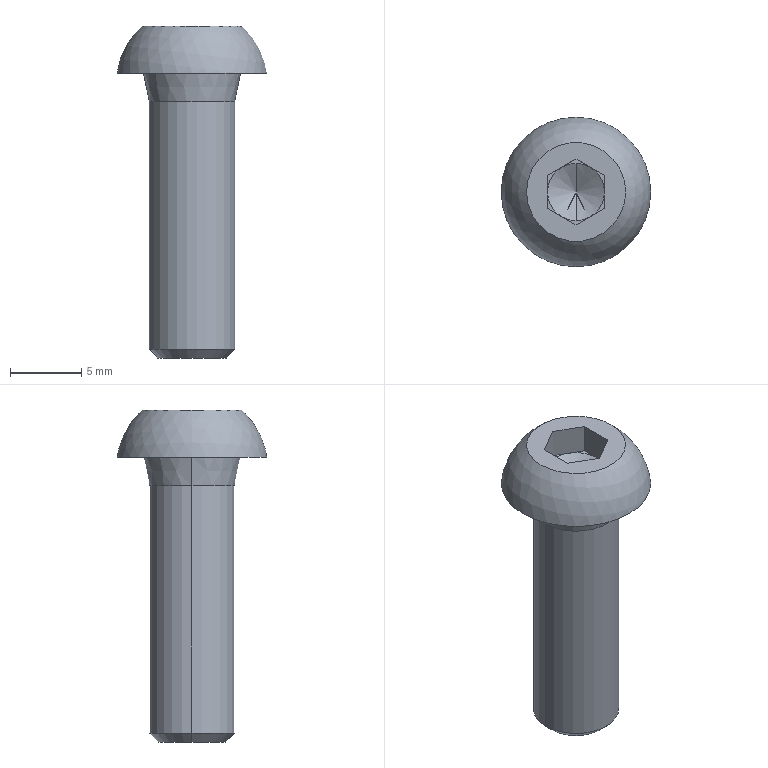Part | SolidWorks | features BaseBody 1 | 1 solid | 24 faces | box 10.5 x 10.5 x 23.3 mm | volume 760.564 mm3 | plane 15 | cone 6 | cylinder 2 | sphere 1 | commonest cylinder face diameters 6 x2
STEP:
#1=CARTESIAN_POINT('',(3.,0.,-17.387));
#2=VERTEX_POINT('',#1);
#3=CARTESIAN_POINT('',(-3.,0.,-17.387));
#4=VERTEX_POINT('',#3);
#5=CARTESIAN_POINT('',(0.,0.,-17.387));
#6=DIRECTION('',(0.,0.,1.));
#7=DIRECTION('',(1.,0.,0.));
#8=AXIS2_PLACEMENT_3D('',#5,#6,#7);
#9=CIRCLE('',#8,3.);
#10=EDGE_CURVE('',#2,#4,#9,.T.);
#11=ORIENTED_EDGE('',*,*,#10,.T.);
#12=CARTESIAN_POINT('',(-3.,0.,0.));
#13=VERTEX_POINT('',#12);
#14=CARTESIAN_POINT('',(-3.,0.,-18.));
#15=DIRECTION('',(0.,0.,1.));
#16=VECTOR('',#15,1000.);
#17=LINE('',#14,#16);
#18=EDGE_CURVE('',#4,#13,#17,.T.);
#19=ORIENTED_EDGE('',*,*,#18,.T.);
#20=CARTESIAN_POINT('',(3.,0.,0.));
#21=VERTEX_POINT('',#20);
#22=CARTESIAN_POINT('',(0.,0.,0.));
#23=DIRECTION('',(0.,0.,-1.));
#24=DIRECTION('',(1.,0.,0.));
#25=AXIS2_PLACEMENT_3D('',#22,#23,#24);
#26=CIRCLE('',#25,3.);
#27=EDGE_CURVE('',#13,#21,#26,.T.);
#28=ORIENTED_EDGE('',*,*,#27,.T.);
#29=CARTESIAN_POINT('',(3.,0.,-18.));
#30=DIRECTION('',(0.,0.,1.));
#31=VECTOR('',#30,1000.);
#32=LINE('',#29,#31);
#33=EDGE_CURVE('',#2,#21,#32,.T.);
#34=ORIENTED_EDGE('',*,*,#33,.F.);
#35=EDGE_LOOP('',(#11,#19,#28,#34));
#36=FACE_OUTER_BOUND('',#35,.T.);
#37=CARTESIAN_POINT('',(0.,0.,-18.));
#38=DIRECTION('',(0.,0.,1.));
#39=DIRECTION('',(1.,0.,0.));
#40=AXIS2_PLACEMENT_3D('',#37,#38,#39);
#41=CYLINDRICAL_SURFACE('',#40,3.);
#42=ADVANCED_FACE('',(#36),#41,.T.);
#43=ORIENTED_EDGE('',*,*,#27,.F.);
#44=CARTESIAN_POINT('',(-3.4,0.,2.));
#45=VERTEX_POINT('',#44);
#46=CARTESIAN_POINT('',(-3.4,0.,2.));
#47=DIRECTION('',(-0.1961,0.,0.9806));
#48=VECTOR('',#47,1000.);
#49=LINE('',#46,#48);
#50=EDGE_CURVE('',#13,#45,#49,.T.);
#51=ORIENTED_EDGE('',*,*,#50,.T.);
#52=CARTESIAN_POINT('',(3.4,0.,2.));
#53=VERTEX_POINT('',#52);
#54=CARTESIAN_POINT('',(0.,0.,2.));
#55=DIRECTION('',(0.,0.,-1.));
#56=DIRECTION('',(1.,0.,0.));
#57=AXIS2_PLACEMENT_3D('',#54,#55,#56);
#58=CIRCLE('',#57,3.4);
#59=EDGE_CURVE('',#45,#53,#58,.T.);
#60=ORIENTED_EDGE('',*,*,#59,.T.);
#61=CARTESIAN_POINT('',(3.4,0.,2.));
#62=DIRECTION('',(0.1961,0.,0.9806));
#63=VECTOR('',#62,1000.);
#64=LINE('',#61,#63);
#65=EDGE_CURVE('',#21,#53,#64,.T.);
#66=ORIENTED_EDGE('',*,*,#65,.F.);
#67=EDGE_LOOP('',(#43,#51,#60,#66));
#68=FACE_OUTER_BOUND('',#67,.T.);
#69=CARTESIAN_POINT('',(0.,0.,2.));
#70=DIRECTION('',(0.,0.,1.));
#71=DIRECTION('',(1.,0.,0.));
#72=AXIS2_PLACEMENT_3D('',#69,#70,#71);
#73=CONICAL_SURFACE('',#72,3.4,0.1974);
#74=ADVANCED_FACE('',(#68),#73,.T.);
#75=CARTESIAN_POINT('',(2.386,0.,-18.));
#76=VERTEX_POINT('',#75);
#77=CARTESIAN_POINT('',(-2.386,0.,-18.));
#78=VERTEX_POINT('',#77);
#79=CARTESIAN_POINT('',(0.,0.,-18.));
#80=DIRECTION('',(0.,0.,1.));
#81=DIRECTION('',(1.,0.,0.));
#82=AXIS2_PLACEMENT_3D('',#79,#80,#81);
#83=CIRCLE('',#82,2.386);
#84=EDGE_CURVE('',#76,#78,#83,.T.);
#85=ORIENTED_EDGE('',*,*,#84,.T.);
#86=CARTESIAN_POINT('',(-3.,0.,-17.387));
#87=DIRECTION('',(-0.7071,0.,0.7071));
#88=VECTOR('',#87,1000.);
#89=LINE('',#86,#88);
#90=EDGE_CURVE('',#78,#4,#89,.T.);
#91=ORIENTED_EDGE('',*,*,#90,.T.);
#92=ORIENTED_EDGE('',*,*,#10,.F.);
#93=CARTESIAN_POINT('',(3.,0.,-17.387));
#94=DIRECTION('',(0.7071,0.,0.7071));
#95=VECTOR('',#94,1000.);
#96=LINE('',#93,#95);
#97=EDGE_CURVE('',#76,#2,#96,.T.);
#98=ORIENTED_EDGE('',*,*,#97,.F.);
#99=EDGE_LOOP('',(#85,#91,#92,#98));
#100=FACE_OUTER_BOUND('',#99,.T.);
#101=CARTESIAN_POINT('',(0.,0.,-17.387));
#102=DIRECTION('',(0.,0.,1.));
#103=DIRECTION('',(1.,0.,0.));
#104=AXIS2_PLACEMENT_3D('',#101,#102,#103);
#105=CONICAL_SURFACE('',#104,3.,0.7854);
#106=ADVANCED_FACE('',(#100),#105,.T.);
#107=CARTESIAN_POINT('',(0.,0.,2.065));
#108=VERTEX_POINT('',#107);
#109=CARTESIAN_POINT('',(0.,-2.,3.22));
#110=VERTEX_POINT('',#109);
#111=CARTESIAN_POINT('',(0.,-2.,3.22));
#112=DIRECTION('',(0.,-0.866,0.5));
#113=VECTOR('',#112,1000.);
#114=LINE('',#111,#113);
#115=EDGE_CURVE('',#108,#110,#114,.T.);
#116=ORIENTED_EDGE('',*,*,#115,.F.);
#117=CARTESIAN_POINT('',(0.,2.,3.22));
#118=VERTEX_POINT('',#117);
#119=CARTESIAN_POINT('',(0.,2.,3.22));
#120=DIRECTION('',(0.,0.866,0.5));
#121=VECTOR('',#120,1000.);
#122=LINE('',#119,#121);
#123=EDGE_CURVE('',#108,#118,#122,.T.);
#124=ORIENTED_EDGE('',*,*,#123,.T.);
#125=CARTESIAN_POINT('',(-1.,1.732,3.22));
#126=VERTEX_POINT('',#125);
#127=CARTESIAN_POINT('',(0.,0.,3.22));
#128=DIRECTION('',(0.,0.,-1.));
#129=DIRECTION('',(0.,-1.,0.));
#130=AXIS2_PLACEMENT_3D('',#127,#128,#129);
#131=CIRCLE('',#130,2.);
#132=EDGE_CURVE('',#126,#118,#131,.T.);
#133=ORIENTED_EDGE('',*,*,#132,.F.);
#134=CARTESIAN_POINT('',(-2.,0.,3.22));
#135=VERTEX_POINT('',#134);
#136=CARTESIAN_POINT('',(0.,0.,3.22));
#137=DIRECTION('',(0.,0.,-1.));
#138=DIRECTION('',(0.,-1.,0.));
#139=AXIS2_PLACEMENT_3D('',#136,#137,#138);
#140=CIRCLE('',#139,2.);
#141=EDGE_CURVE('',#135,#126,#140,.T.);
#142=ORIENTED_EDGE('',*,*,#141,.F.);
#143=CARTESIAN_POINT('',(-1.,-1.732,3.22));
#144=VERTEX_POINT('',#143);
#145=CARTESIAN_POINT('',(0.,0.,3.22));
#146=DIRECTION('',(0.,0.,-1.));
#147=DIRECTION('',(0.,-1.,0.));
#148=AXIS2_PLACEMENT_3D('',#145,#146,#147);
#149=CIRCLE('',#148,2.);
#150=EDGE_CURVE('',#144,#135,#149,.T.);
#151=ORIENTED_EDGE('',*,*,#150,.F.);
#152=CARTESIAN_POINT('',(0.,0.,3.22));
#153=DIRECTION('',(0.,0.,-1.));
#154=DIRECTION('',(0.,-1.,0.));
#155=AXIS2_PLACEMENT_3D('',#152,#153,#154);
#156=CIRCLE('',#155,2.);
#157=EDGE_CURVE('',#110,#144,#156,.T.);
#158=ORIENTED_EDGE('',*,*,#157,.F.);
#159=EDGE_LOOP('',(#116,#124,#133,#142,#151,#158));
#160=FACE_OUTER_BOUND('',#159,.T.);
#161=CARTESIAN_POINT('',(0.,0.,3.22));
#162=DIRECTION('',(0.,0.,1.));
#163=DIRECTION('',(0.,-1.,0.));
#164=AXIS2_PLACEMENT_3D('',#161,#162,#163);
#165=CONICAL_SURFACE('',#164,2.,1.047);
#166=ADVANCED_FACE('',(#160),#165,.F.);
#167=ORIENTED_EDGE('',*,*,#18,.F.);
#168=CARTESIAN_POINT('',(0.,0.,-17.387));
#169=DIRECTION('',(0.,0.,1.));
#170=DIRECTION('',(1.,0.,0.));
#171=AXIS2_PLACEMENT_3D('',#168,#169,#170);
#172=CIRCLE('',#171,3.);
#173=EDGE_CURVE('',#4,#2,#172,.T.);
#174=ORIENTED_EDGE('',*,*,#173,.T.);
#175=ORIENTED_EDGE('',*,*,#33,.T.);
#176=CARTESIAN_POINT('',(0.,0.,0.));
#177=DIRECTION('',(0.,0.,-1.));
#178=DIRECTION('',(1.,0.,0.));
#179=AXIS2_PLACEMENT_3D('',#176,#177,#178);
#180=CIRCLE('',#179,3.);
#181=EDGE_CURVE('',#21,#13,#180,.T.);
#182=ORIENTED_EDGE('',*,*,#181,.T.);
#183=EDGE_LOOP('',(#167,#174,#175,#182));
#184=FACE_OUTER_BOUND('',#183,.T.);
#185=CARTESIAN_POINT('',(0.,0.,-18.));
#186=DIRECTION('',(0.,0.,1.));
#187=DIRECTION('',(1.,0.,0.));
#188=AXIS2_PLACEMENT_3D('',#185,#186,#187);
#189=CYLINDRICAL_SURFACE('',#188,3.);
#190=ADVANCED_FACE('',(#184),#189,.T.);
#191=ORIENTED_EDGE('',*,*,#50,.F.);
#192=ORIENTED_EDGE('',*,*,#181,.F.);
#193=ORIENTED_EDGE('',*,*,#65,.T.);
#194=CARTESIAN_POINT('',(0.,0.,2.));
#195=DIRECTION('',(0.,0.,-1.));
#196=DIRECTION('',(1.,0.,0.));
#197=AXIS2_PLACEMENT_3D('',#194,#195,#196);
#198=CIRCLE('',#197,3.4);
#199=EDGE_CURVE('',#53,#45,#198,.T.);
#200=ORIENTED_EDGE('',*,*,#199,.T.);
#201=EDGE_LOOP('',(#191,#192,#193,#200));
#202=FACE_OUTER_BOUND('',#201,.T.);
#203=CARTESIAN_POINT('',(0.,0.,2.));
#204=DIRECTION('',(0.,0.,1.));
#205=DIRECTION('',(1.,0.,0.));
#206=AXIS2_PLACEMENT_3D('',#203,#204,#205);
#207=CONICAL_SURFACE('',#206,3.4,0.1974);
#208=ADVANCED_FACE('',(#202),#207,.T.);
#209=ORIENTED_EDGE('',*,*,#90,.F.);
#210=CARTESIAN_POINT('',(0.,0.,-18.));
#211=DIRECTION('',(0.,0.,1.));
#212=DIRECTION('',(1.,0.,0.));
#213=AXIS2_PLACEMENT_3D('',#210,#211,#212);
#214=CIRCLE('',#213,2.386);
#215=EDGE_CURVE('',#78,#76,#214,.T.);
#216=ORIENTED_EDGE('',*,*,#215,.T.);
#217=ORIENTED_EDGE('',*,*,#97,.T.);
#218=ORIENTED_EDGE('',*,*,#173,.F.);
#219=EDGE_LOOP('',(#209,#216,#217,#218));
#220=FACE_OUTER_BOUND('',#219,.T.);
#221=CARTESIAN_POINT('',(0.,0.,-17.387));
#222=DIRECTION('',(0.,0.,1.));
#223=DIRECTION('',(1.,0.,0.));
#224=AXIS2_PLACEMENT_3D('',#221,#222,#223);
#225=CONICAL_SURFACE('',#224,3.,0.7854);
#226=ADVANCED_FACE('',(#220),#225,.T.);
#227=CARTESIAN_POINT('',(5.25,0.,2.));
#228=VERTEX_POINT('',#227);
#229=CARTESIAN_POINT('',(-5.25,0.,2.));
#230=VERTEX_POINT('',#229);
#231=CARTESIAN_POINT('',(0.,0.,2.));
#232=DIRECTION('',(0.,0.,1.));
#233=DIRECTION('',(1.,0.,0.));
#234=AXIS2_PLACEMENT_3D('',#231,#232,#233);
#235=CIRCLE('',#234,5.25);
#236=EDGE_CURVE('',#228,#230,#235,.T.);
#237=ORIENTED_EDGE('',*,*,#236,.F.);
#238=CARTESIAN_POINT('',(0.,0.,2.));
#239=DIRECTION('',(0.,0.,1.));
#240=DIRECTION('',(1.,0.,0.));
#241=AXIS2_PLACEMENT_3D('',#238,#239,#240);
#242=CIRCLE('',#241,5.25);
#243=EDGE_CURVE('',#230,#228,#242,.T.);
#244=ORIENTED_EDGE('',*,*,#243,.F.);
#245=EDGE_LOOP('',(#237,#244));
#246=FACE_OUTER_BOUND('',#245,.T.);
#247=ORIENTED_EDGE('',*,*,#199,.F.);
#248=ORIENTED_EDGE('',*,*,#59,.F.);
#249=EDGE_LOOP('',(#247,#248));
#250=FACE_BOUND('',#249,.T.);
#251=CARTESIAN_POINT('',(0.,5.25,2.));
#252=DIRECTION('',(0.,0.,1.));
#253=DIRECTION('',(1.,0.,0.));
#254=AXIS2_PLACEMENT_3D('',#251,#252,#253);
#255=PLANE('',#254);
#256=ADVANCED_FACE('',(#246,#250),#255,.F.);
#257=ORIENTED_EDGE('',*,*,#84,.F.);
#258=ORIENTED_EDGE('',*,*,#215,.F.);
#259=EDGE_LOOP('',(#257,#258));
#260=FACE_OUTER_BOUND('',#259,.T.);
#261=CARTESIAN_POINT('',(3.,0.,-18.));
#262=DIRECTION('',(0.,0.,-1.));
#263=DIRECTION('',(-1.,0.,0.));
#264=AXIS2_PLACEMENT_3D('',#261,#262,#263);
#265=PLANE('',#264);
#266=ADVANCED_FACE('',(#260),#265,.T.);
#267=CARTESIAN_POINT('',(-3.472,0.,5.3));
#268=VERTEX_POINT('',#267);
#269=CARTESIAN_POINT('',(3.472,0.,5.3));
#270=VERTEX_POINT('',#269);
#271=CARTESIAN_POINT('',(0.,0.,5.3));
#272=DIRECTION('',(0.,0.,-1.));
#273=DIRECTION('',(-1.,0.,0.));
#274=AXIS2_PLACEMENT_3D('',#271,#272,#273);
#275=CIRCLE('',#274,3.472);
#276=EDGE_CURVE('',#268,#270,#275,.T.);
#277=ORIENTED_EDGE('',*,*,#276,.T.);
#278=CARTESIAN_POINT('',(0.,0.,5.3));
#279=DIRECTION('',(0.,0.,-1.));
#280=DIRECTION('',(-1.,0.,0.));
#281=AXIS2_PLACEMENT_3D('',#278,#279,#280);
#282=CIRCLE('',#281,3.472);
#283=EDGE_CURVE('',#270,#268,#282,.T.);
#284=ORIENTED_EDGE('',*,*,#283,.T.);
#285=EDGE_LOOP('',(#277,#284));
#286=FACE_BOUND('',#285,.T.);
#287=ORIENTED_EDGE('',*,*,#236,.T.);
#288=ORIENTED_EDGE('',*,*,#243,.T.);
#289=EDGE_LOOP('',(#287,#288));
#290=FACE_OUTER_BOUND('',#289,.T.);
#291=CARTESIAN_POINT('',(0.,0.,1.3));
#292=DIRECTION('',(0.115,0.,0.9934));
#293=DIRECTION('',(-0.9934,0.,0.115));
#294=AXIS2_PLACEMENT_3D('',#291,#292,#293);
#295=SPHERICAL_SURFACE('',#294,5.296);
#296=ADVANCED_FACE('',(#286,#290),#295,.T.);
#297=ORIENTED_EDGE('',*,*,#276,.F.);
#298=ORIENTED_EDGE('',*,*,#283,.F.);
#299=EDGE_LOOP('',(#297,#298));
#300=FACE_OUTER_BOUND('',#299,.T.);
#301=CARTESIAN_POINT('',(2.,-1.155,5.3));
#302=VERTEX_POINT('',#301);
#303=CARTESIAN_POINT('',(2.,1.155,5.3));
#304=VERTEX_POINT('',#303);
#305=CARTESIAN_POINT('',(2.,0.,5.3));
#306=DIRECTION('',(0.,1.,0.));
#307=VECTOR('',#306,1000.);
#308=LINE('',#305,#307);
#309=EDGE_CURVE('',#302,#304,#308,.T.);
#310=ORIENTED_EDGE('',*,*,#309,.F.);
#311=CARTESIAN_POINT('',(0.,-2.309,5.3));
#312=VERTEX_POINT('',#311);
#313=CARTESIAN_POINT('',(0.,-2.309,5.3));
#314=DIRECTION('',(0.866,0.5,0.));
#315=VECTOR('',#314,1000.);
#316=LINE('',#313,#315);
#317=EDGE_CURVE('',#312,#302,#316,.T.);
#318=ORIENTED_EDGE('',*,*,#317,.F.);
#319=CARTESIAN_POINT('',(-2.,-1.155,5.3));
#320=VERTEX_POINT('',#319);
#321=CARTESIAN_POINT('',(-2.,-1.155,5.3));
#322=DIRECTION('',(0.866,-0.5,0.));
#323=VECTOR('',#322,1000.);
#324=LINE('',#321,#323);
#325=EDGE_CURVE('',#320,#312,#324,.T.);
#326=ORIENTED_EDGE('',*,*,#325,.F.);
#327=CARTESIAN_POINT('',(-2.,1.155,5.3));
#328=VERTEX_POINT('',#327);
#329=CARTESIAN_POINT('',(-2.,0.,5.3));
#330=DIRECTION('',(0.,-1.,0.));
#331=VECTOR('',#330,1000.);
#332=LINE('',#329,#331);
#333=EDGE_CURVE('',#328,#320,#332,.T.);
#334=ORIENTED_EDGE('',*,*,#333,.F.);
#335=CARTESIAN_POINT('',(0.,2.309,5.3));
#336=VERTEX_POINT('',#335);
#337=CARTESIAN_POINT('',(0.,2.309,5.3));
#338=DIRECTION('',(-0.866,-0.5,0.));
#339=VECTOR('',#338,1000.);
#340=LINE('',#337,#339);
#341=EDGE_CURVE('',#336,#328,#340,.T.);
#342=ORIENTED_EDGE('',*,*,#341,.F.);
#343=CARTESIAN_POINT('',(2.,1.155,5.3));
#344=DIRECTION('',(-0.866,0.5,0.));
#345=VECTOR('',#344,1000.);
#346=LINE('',#343,#345);
#347=EDGE_CURVE('',#304,#336,#346,.T.);
#348=ORIENTED_EDGE('',*,*,#347,.F.);
#349=EDGE_LOOP('',(#310,#318,#326,#334,#342,#348));
#350=FACE_BOUND('',#349,.T.);
#351=CARTESIAN_POINT('',(0.,0.,5.3));
#352=DIRECTION('',(0.,0.,-1.));
#353=DIRECTION('',(-1.,0.,0.));
#354=AXIS2_PLACEMENT_3D('',#351,#352,#353);
#355=PLANE('',#354);
#356=ADVANCED_FACE('',(#300,#350),#355,.F.);
#357=CARTESIAN_POINT('',(0.,2.309,3.22));
#358=VERTEX_POINT('',#357);
#359=CARTESIAN_POINT('',(0.,2.309,3.22));
#360=DIRECTION('',(0.,0.,1.));
#361=VECTOR('',#360,1000.);
#362=LINE('',#359,#361);
#363=EDGE_CURVE('',#358,#336,#362,.T.);
#364=ORIENTED_EDGE('',*,*,#363,.F.);
#365=CARTESIAN_POINT('',(1.,1.732,3.22));
#366=VERTEX_POINT('',#365);
#367=CARTESIAN_POINT('',(2.,1.155,3.22));
#368=DIRECTION('',(-0.866,0.5,0.));
#369=VECTOR('',#368,1000.);
#370=LINE('',#367,#369);
#371=EDGE_CURVE('',#366,#358,#370,.T.);
#372=ORIENTED_EDGE('',*,*,#371,.F.);
#373=CARTESIAN_POINT('',(2.,1.155,3.22));
#374=VERTEX_POINT('',#373);
#375=CARTESIAN_POINT('',(2.,1.155,3.22));
#376=DIRECTION('',(-0.866,0.5,0.));
#377=VECTOR('',#376,1000.);
#378=LINE('',#375,#377);
#379=EDGE_CURVE('',#374,#366,#378,.T.);
#380=ORIENTED_EDGE('',*,*,#379,.F.);
#381=CARTESIAN_POINT('',(2.,1.155,3.22));
#382=DIRECTION('',(0.,0.,-1.));
#383=VECTOR('',#382,1000.);
#384=LINE('',#381,#383);
#385=EDGE_CURVE('',#304,#374,#384,.T.);
#386=ORIENTED_EDGE('',*,*,#385,.F.);
#387=ORIENTED_EDGE('',*,*,#347,.T.);
#388=EDGE_LOOP('',(#364,#372,#380,#386,#387));
#389=FACE_OUTER_BOUND('',#388,.T.);
#390=CARTESIAN_POINT('',(2.,1.155,3.22));
#391=DIRECTION('',(0.5,0.866,0.));
#392=DIRECTION('',(-0.866,0.5,0.));
#393=AXIS2_PLACEMENT_3D('',#390,#391,#392);
#394=PLANE('',#393);
#395=ADVANCED_FACE('',(#389),#394,.F.);
#396=ORIENTED_EDGE('',*,*,#385,.T.);
#397=CARTESIAN_POINT('',(2.,0.,3.22));
#398=VERTEX_POINT('',#397);
#399=CARTESIAN_POINT('',(2.,0.,3.22));
#400=DIRECTION('',(0.,1.,0.));
#401=VECTOR('',#400,1000.);
#402=LINE('',#399,#401);
#403=EDGE_CURVE('',#398,#374,#402,.T.);
#404=ORIENTED_EDGE('',*,*,#403,.F.);
#405=CARTESIAN_POINT('',(2.,-1.155,3.22));
#406=VERTEX_POINT('',#405);
#407=CARTESIAN_POINT('',(2.,0.,3.22));
#408=DIRECTION('',(0.,1.,0.));
#409=VECTOR('',#408,1000.);
#410=LINE('',#407,#409);
#411=EDGE_CURVE('',#406,#398,#410,.T.);
#412=ORIENTED_EDGE('',*,*,#411,.F.);
#413=CARTESIAN_POINT('',(2.,-1.155,3.22));
#414=DIRECTION('',(0.,0.,-1.));
#415=VECTOR('',#414,1000.);
#416=LINE('',#413,#415);
#417=EDGE_CURVE('',#302,#406,#416,.T.);
#418=ORIENTED_EDGE('',*,*,#417,.F.);
#419=ORIENTED_EDGE('',*,*,#309,.T.);
#420=EDGE_LOOP('',(#396,#404,#412,#418,#419));
#421=FACE_OUTER_BOUND('',#420,.T.);
#422=CARTESIAN_POINT('',(2.,-1.155,3.22));
#423=DIRECTION('',(1.,0.,0.));
#424=DIRECTION('',(0.,0.,-1.));
#425=AXIS2_PLACEMENT_3D('',#422,#423,#424);
#426=PLANE('',#425);
#427=ADVANCED_FACE('',(#421),#426,.F.);
#428=ORIENTED_EDGE('',*,*,#417,.T.);
#429=CARTESIAN_POINT('',(1.,-1.732,3.22));
#430=VERTEX_POINT('',#429);
#431=CARTESIAN_POINT('',(1.,-1.732,3.22));
#432=DIRECTION('',(0.866,0.5,0.));
#433=VECTOR('',#432,1000.);
#434=LINE('',#431,#433);
#435=EDGE_CURVE('',#430,#406,#434,.T.);
#436=ORIENTED_EDGE('',*,*,#435,.F.);
#437=CARTESIAN_POINT('',(0.,-2.309,3.22));
#438=VERTEX_POINT('',#437);
#439=CARTESIAN_POINT('',(0.,-2.309,3.22));
#440=DIRECTION('',(0.866,0.5,0.));
#441=VECTOR('',#440,1000.);
#442=LINE('',#439,#441);
#443=EDGE_CURVE('',#438,#430,#442,.T.);
#444=ORIENTED_EDGE('',*,*,#443,.F.);
#445=CARTESIAN_POINT('',(0.,-2.309,3.22));
#446=DIRECTION('',(0.,0.,-1.));
#447=VECTOR('',#446,1000.);
#448=LINE('',#445,#447);
#449=EDGE_CURVE('',#312,#438,#448,.T.);
#450=ORIENTED_EDGE('',*,*,#449,.F.);
#451=ORIENTED_EDGE('',*,*,#317,.T.);
#452=EDGE_LOOP('',(#428,#436,#444,#450,#451));
#453=FACE_OUTER_BOUND('',#452,.T.);
#454=CARTESIAN_POINT('',(0.,-2.309,3.22));
#455=DIRECTION('',(0.5,-0.866,0.));
#456=DIRECTION('',(0.866,0.5,0.));
#457=AXIS2_PLACEMENT_3D('',#454,#455,#456);
#458=PLANE('',#457);
#459=ADVANCED_FACE('',(#453),#458,.F.);
#460=ORIENTED_EDGE('',*,*,#449,.T.);
#461=CARTESIAN_POINT('',(-2.,-1.155,3.22));
#462=DIRECTION('',(0.866,-0.5,0.));
#463=VECTOR('',#462,1000.);
#464=LINE('',#461,#463);
#465=EDGE_CURVE('',#144,#438,#464,.T.);
#466=ORIENTED_EDGE('',*,*,#465,.F.);
#467=CARTESIAN_POINT('',(-2.,-1.155,3.22));
#468=VERTEX_POINT('',#467);
#469=CARTESIAN_POINT('',(-2.,-1.155,3.22));
#470=DIRECTION('',(0.866,-0.5,0.));
#471=VECTOR('',#470,1000.);
#472=LINE('',#469,#471);
#473=EDGE_CURVE('',#468,#144,#472,.T.);
#474=ORIENTED_EDGE('',*,*,#473,.F.);
#475=CARTESIAN_POINT('',(-2.,-1.155,3.22));
#476=DIRECTION('',(0.,0.,-1.));
#477=VECTOR('',#476,1000.);
#478=LINE('',#475,#477);
#479=EDGE_CURVE('',#320,#468,#478,.T.);
#480=ORIENTED_EDGE('',*,*,#479,.F.);
#481=ORIENTED_EDGE('',*,*,#325,.T.);
#482=EDGE_LOOP('',(#460,#466,#474,#480,#481));
#483=FACE_OUTER_BOUND('',#482,.T.);
#484=CARTESIAN_POINT('',(-2.,-1.155,3.22));
#485=DIRECTION('',(-0.5,-0.866,0.));
#486=DIRECTION('',(0.866,-0.5,0.));
#487=AXIS2_PLACEMENT_3D('',#484,#485,#486);
#488=PLANE('',#487);
#489=ADVANCED_FACE('',(#483),#488,.F.);
#490=ORIENTED_EDGE('',*,*,#479,.T.);
#491=CARTESIAN_POINT('',(-2.,0.,3.22));
#492=DIRECTION('',(0.,-1.,0.));
#493=VECTOR('',#492,1000.);
#494=LINE('',#491,#493);
#495=EDGE_CURVE('',#135,#468,#494,.T.);
#496=ORIENTED_EDGE('',*,*,#495,.F.);
#497=CARTESIAN_POINT('',(-2.,1.155,3.22));
#498=VERTEX_POINT('',#497);
#499=CARTESIAN_POINT('',(-2.,0.,3.22));
#500=DIRECTION('',(0.,-1.,0.));
#501=VECTOR('',#500,1000.);
#502=LINE('',#499,#501);
#503=EDGE_CURVE('',#498,#135,#502,.T.);
#504=ORIENTED_EDGE('',*,*,#503,.F.);
#505=CARTESIAN_POINT('',(-2.,1.155,3.22));
#506=DIRECTION('',(0.,0.,-1.));
#507=VECTOR('',#506,1000.);
#508=LINE('',#505,#507);
#509=EDGE_CURVE('',#328,#498,#508,.T.);
#510=ORIENTED_EDGE('',*,*,#509,.F.);
#511=ORIENTED_EDGE('',*,*,#333,.T.);
#512=EDGE_LOOP('',(#490,#496,#504,#510,#511));
#513=FACE_OUTER_BOUND('',#512,.T.);
#514=CARTESIAN_POINT('',(-2.,1.155,3.22));
#515=DIRECTION('',(-1.,0.,0.));
#516=DIRECTION('',(0.,0.,1.));
#517=AXIS2_PLACEMENT_3D('',#514,#515,#516);
#518=PLANE('',#517);
#519=ADVANCED_FACE('',(#513),#518,.F.);
#520=ORIENTED_EDGE('',*,*,#509,.T.);
#521=CARTESIAN_POINT('',(0.,2.309,3.22));
#522=DIRECTION('',(-0.866,-0.5,0.));
#523=VECTOR('',#522,1000.);
#524=LINE('',#521,#523);
#525=EDGE_CURVE('',#126,#498,#524,.T.);
#526=ORIENTED_EDGE('',*,*,#525,.F.);
#527=CARTESIAN_POINT('',(0.,2.309,3.22));
#528=DIRECTION('',(-0.866,-0.5,0.));
#529=VECTOR('',#528,1000.);
#530=LINE('',#527,#529);
#531=EDGE_CURVE('',#358,#126,#530,.T.);
#532=ORIENTED_EDGE('',*,*,#531,.F.);
#533=ORIENTED_EDGE('',*,*,#363,.T.);
#534=ORIENTED_EDGE('',*,*,#341,.T.);
#535=EDGE_LOOP('',(#520,#526,#532,#533,#534));
#536=FACE_OUTER_BOUND('',#535,.T.);
#537=CARTESIAN_POINT('',(0.,2.309,3.22));
#538=DIRECTION('',(-0.5,0.866,0.));
#539=DIRECTION('',(-0.866,-0.5,0.));
#540=AXIS2_PLACEMENT_3D('',#537,#538,#539);
#541=PLANE('',#540);
#542=ADVANCED_FACE('',(#536),#541,.F.);
#543=ORIENTED_EDGE('',*,*,#132,.T.);
#544=CARTESIAN_POINT('',(0.,0.,3.22));
#545=DIRECTION('',(0.,0.,-1.));
#546=DIRECTION('',(0.,-1.,0.));
#547=AXIS2_PLACEMENT_3D('',#544,#545,#546);
#548=CIRCLE('',#547,2.);
#549=EDGE_CURVE('',#118,#366,#548,.T.);
#550=ORIENTED_EDGE('',*,*,#549,.T.);
#551=ORIENTED_EDGE('',*,*,#371,.T.);
#552=ORIENTED_EDGE('',*,*,#531,.T.);
#553=EDGE_LOOP('',(#543,#550,#551,#552));
#554=FACE_OUTER_BOUND('',#553,.T.);
#555=CARTESIAN_POINT('',(0.,0.,3.22));
#556=DIRECTION('',(0.,0.,1.));
#557=DIRECTION('',(1.,0.,0.));
#558=AXIS2_PLACEMENT_3D('',#555,#556,#557);
#559=PLANE('',#558);
#560=ADVANCED_FACE('',(#554),#559,.T.);
#561=CARTESIAN_POINT('',(0.,0.,3.22));
#562=DIRECTION('',(0.,0.,-1.));
#563=DIRECTION('',(0.,-1.,0.));
#564=AXIS2_PLACEMENT_3D('',#561,#562,#563);
#565=CIRCLE('',#564,2.);
#566=EDGE_CURVE('',#430,#110,#565,.T.);
#567=ORIENTED_EDGE('',*,*,#566,.T.);
#568=ORIENTED_EDGE('',*,*,#157,.T.);
#569=ORIENTED_EDGE('',*,*,#465,.T.);
#570=ORIENTED_EDGE('',*,*,#443,.T.);
#571=EDGE_LOOP('',(#567,#568,#569,#570));
#572=FACE_OUTER_BOUND('',#571,.T.);
#573=CARTESIAN_POINT('',(0.,0.,3.22));
#574=DIRECTION('',(0.,0.,1.));
#575=DIRECTION('',(1.,0.,0.));
#576=AXIS2_PLACEMENT_3D('',#573,#574,#575);
#577=PLANE('',#576);
#578=ADVANCED_FACE('',(#572),#577,.T.);
#579=ORIENTED_EDGE('',*,*,#141,.T.);
#580=ORIENTED_EDGE('',*,*,#525,.T.);
#581=ORIENTED_EDGE('',*,*,#503,.T.);
#582=EDGE_LOOP('',(#579,#580,#581));
#583=FACE_OUTER_BOUND('',#582,.T.);
#584=CARTESIAN_POINT('',(0.,0.,3.22));
#585=DIRECTION('',(0.,0.,1.));
#586=DIRECTION('',(1.,0.,0.));
#587=AXIS2_PLACEMENT_3D('',#584,#585,#586);
#588=PLANE('',#587);
#589=ADVANCED_FACE('',(#583),#588,.T.);
#590=ORIENTED_EDGE('',*,*,#123,.F.);
#591=ORIENTED_EDGE('',*,*,#115,.T.);
#592=ORIENTED_EDGE('',*,*,#566,.F.);
#593=CARTESIAN_POINT('',(0.,0.,3.22));
#594=DIRECTION('',(0.,0.,-1.));
#595=DIRECTION('',(0.,-1.,0.));
#596=AXIS2_PLACEMENT_3D('',#593,#594,#595);
#597=CIRCLE('',#596,2.);
#598=EDGE_CURVE('',#398,#430,#597,.T.);
#599=ORIENTED_EDGE('',*,*,#598,.F.);
#600=CARTESIAN_POINT('',(0.,0.,3.22));
#601=DIRECTION('',(0.,0.,-1.));
#602=DIRECTION('',(0.,-1.,0.));
#603=AXIS2_PLACEMENT_3D('',#600,#601,#602);
#604=CIRCLE('',#603,2.);
#605=EDGE_CURVE('',#366,#398,#604,.T.);
#606=ORIENTED_EDGE('',*,*,#605,.F.);
#607=ORIENTED_EDGE('',*,*,#549,.F.);
#608=EDGE_LOOP('',(#590,#591,#592,#599,#606,#607));
#609=FACE_OUTER_BOUND('',#608,.T.);
#610=CARTESIAN_POINT('',(0.,0.,3.22));
#611=DIRECTION('',(0.,0.,1.));
#612=DIRECTION('',(0.,-1.,0.));
#613=AXIS2_PLACEMENT_3D('',#610,#611,#612);
#614=CONICAL_SURFACE('',#613,2.,1.047);
#615=ADVANCED_FACE('',(#609),#614,.F.);
#616=ORIENTED_EDGE('',*,*,#150,.T.);
#617=ORIENTED_EDGE('',*,*,#495,.T.);
#618=ORIENTED_EDGE('',*,*,#473,.T.);
#619=EDGE_LOOP('',(#616,#617,#618));
#620=FACE_OUTER_BOUND('',#619,.T.);
#621=CARTESIAN_POINT('',(0.,0.,3.22));
#622=DIRECTION('',(0.,0.,1.));
#623=DIRECTION('',(1.,0.,0.));
#624=AXIS2_PLACEMENT_3D('',#621,#622,#623);
#625=PLANE('',#624);
#626=ADVANCED_FACE('',(#620),#625,.T.);
#627=ORIENTED_EDGE('',*,*,#598,.T.);
#628=ORIENTED_EDGE('',*,*,#435,.T.);
#629=ORIENTED_EDGE('',*,*,#411,.T.);
#630=EDGE_LOOP('',(#627,#628,#629));
#631=FACE_OUTER_BOUND('',#630,.T.);
#632=CARTESIAN_POINT('',(0.,0.,3.22));
#633=DIRECTION('',(0.,0.,1.));
#634=DIRECTION('',(1.,0.,0.));
#635=AXIS2_PLACEMENT_3D('',#632,#633,#634);
#636=PLANE('',#635);
#637=ADVANCED_FACE('',(#631),#636,.T.);
#638=ORIENTED_EDGE('',*,*,#605,.T.);
#639=ORIENTED_EDGE('',*,*,#403,.T.);
#640=ORIENTED_EDGE('',*,*,#379,.T.);
#641=EDGE_LOOP('',(#638,#639,#640));
#642=FACE_OUTER_BOUND('',#641,.T.);
#643=CARTESIAN_POINT('',(0.,0.,3.22));
#644=DIRECTION('',(0.,0.,1.));
#645=DIRECTION('',(1.,0.,0.));
#646=AXIS2_PLACEMENT_3D('',#643,#644,#645);
#647=PLANE('',#646);
#648=ADVANCED_FACE('',(#642),#647,.T.);
#649=CLOSED_SHELL('',(#42,#74,#106,#166,#190,#208,#226,#256,#266,#296,#356,#395,#427,#459,#489,#519,#542,#560,#578,#589,#615,#626,#637,#648));
#650=MANIFOLD_SOLID_BREP('',#649);
#651=CARTESIAN_POINT('',(0.,0.,0.));
#652=DIRECTION('',(0.,0.,1.));
#653=DIRECTION('',(1.,0.,0.));
#654=AXIS2_PLACEMENT_3D('',#651,#652,#653);
#655=(LENGTH_UNIT()NAMED_UNIT(*)SI_UNIT(.MILLI.,.METRE.));
#656=UNCERTAINTY_MEASURE_WITH_UNIT(LENGTH_MEASURE(0.00001),#655,'','');
#657=(NAMED_UNIT(*)PLANE_ANGLE_UNIT()SI_UNIT($,.RADIAN.));
#658=(NAMED_UNIT(*)SI_UNIT($,.STERADIAN.)SOLID_ANGLE_UNIT());
#659=(GEOMETRIC_REPRESENTATION_CONTEXT(3)GLOBAL_UNCERTAINTY_ASSIGNED_CONTEXT((#656))GLOBAL_UNIT_ASSIGNED_CONTEXT((#655,#657,#658))REPRESENTATION_CONTEXT('',''));
#660=ADVANCED_BREP_SHAPE_REPRESENTATION('',(#650,#654),#659);